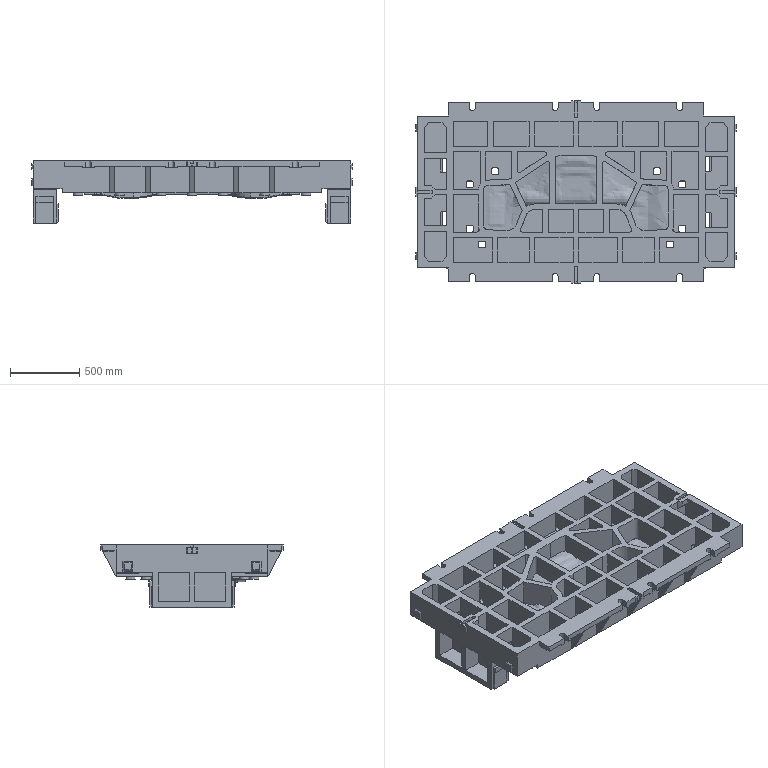Part | NX | features solid 2 | 1 solid | 3403 faces | volume 314962042 mm3 | spline 1558 | plane 996 | cylinder 817 | cone 16 | sphere 16 | commonest cylinder face diameters 9.6 x57 20 x56 14.4 x53 40 x35 8.4 x29 10.4 x27